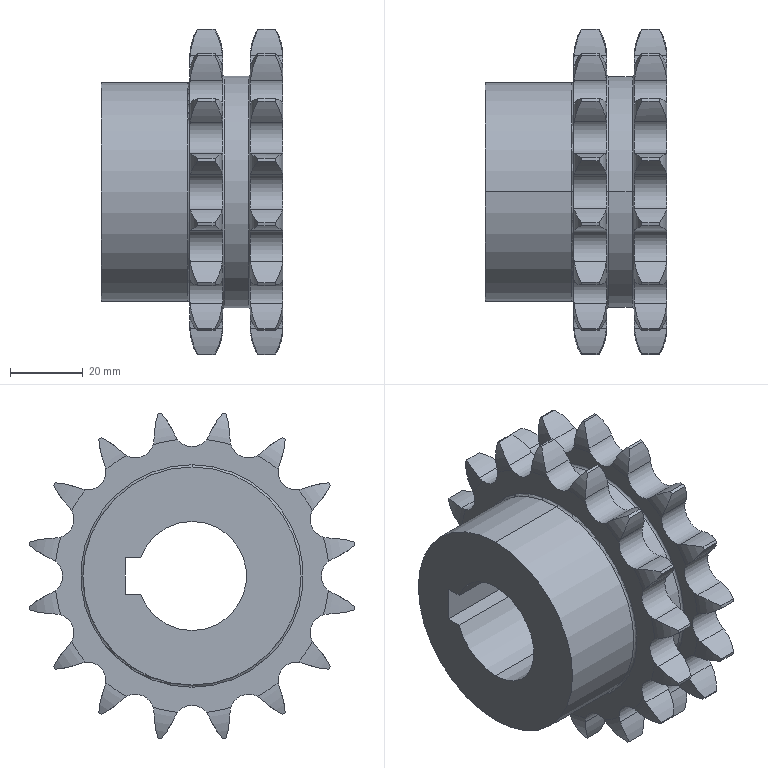Part | STEP file | short pitch roller chain wheel_d_iso_Chain wheel ISO - 16Z 10B-2 --16SB60H50L30.0R1 | 1 solid | 223 faces | box 50.001 x 89.463 x 89.463 mm | volume 141597 mm3 | cylinder 145 | torus 70 | plane 8 | commonest cylinder face diameters 43.891 x64 10.262 x42 91.056 x32 30 x3 60 x2 63.73 x2